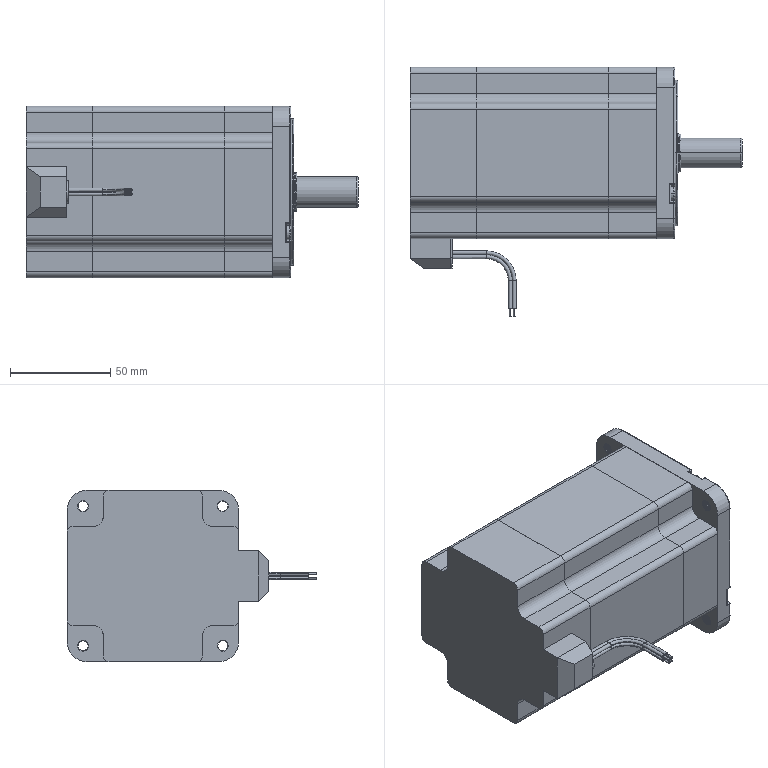Part | SolidWorks | features ICE 14, Fillet 3, CirPattern 2, CombineBodies 1, Extrusion 1, HoleWzd 1, LPattern 1, MoveCopyBody 1, RevCut 1, Sweep 1 | 1 solid | 797 faces | box 165.5 x 124.49 x 85.5 mm | volume 823619 mm3 | cone 482 | plane 146 | cylinder 126 | torus 35 | sphere 8 | commonest cylinder face diameters 1 x36 6 x26 1.9 x20 7 x8 10.02 x8 9 x5